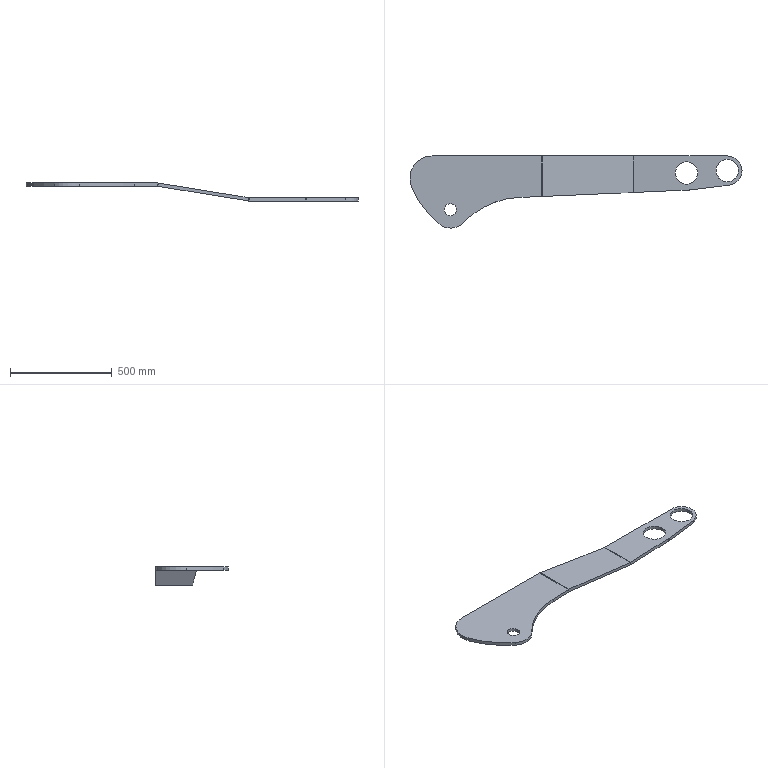Part | SolidWorks | features SM3dBend 2, FlatPattern 1, SMBaseFlange 1, SheetMetal 1 | 1 solid | 34 faces | box 1631 x 354.5 x 88.747 mm | volume 5017835 mm3 | cylinder 17 | plane 15 | spline 2 | commonest cylinder face diameters 60 x4 110 x4 28 x2 144 x2 168 x1 180 x1
STEP:
#1=CARTESIAN_POINT('',(1304.262,192.5,-88.747));
#2=VERTEX_POINT('',#1);
#3=CARTESIAN_POINT('',(1414.262,192.5,-88.747));
#4=VERTEX_POINT('',#3);
#5=CARTESIAN_POINT('',(1359.262,192.5,-88.747));
#6=DIRECTION('',(0.,0.,1.));
#7=DIRECTION('',(1.,0.,0.));
#8=AXIS2_PLACEMENT_3D('',#5,#6,#7);
#9=CIRCLE('',#8,55.);
#10=EDGE_CURVE('',#2,#4,#9,.T.);
#11=ORIENTED_EDGE('',*,*,#10,.F.);
#12=CARTESIAN_POINT('',(1304.262,192.5,-72.747));
#13=VERTEX_POINT('',#12);
#14=CARTESIAN_POINT('',(1304.262,192.5,-88.747));
#15=DIRECTION('',(0.,0.,1.));
#16=VECTOR('',#15,1000.);
#17=LINE('',#14,#16);
#18=EDGE_CURVE('',#2,#13,#17,.T.);
#19=ORIENTED_EDGE('',*,*,#18,.T.);
#20=CARTESIAN_POINT('',(1414.262,192.5,-72.747));
#21=VERTEX_POINT('',#20);
#22=CARTESIAN_POINT('',(1359.262,192.5,-72.747));
#23=DIRECTION('',(0.,0.,1.));
#24=DIRECTION('',(1.,0.,0.));
#25=AXIS2_PLACEMENT_3D('',#22,#23,#24);
#26=CIRCLE('',#25,55.);
#27=EDGE_CURVE('',#13,#21,#26,.T.);
#28=ORIENTED_EDGE('',*,*,#27,.T.);
#29=CARTESIAN_POINT('',(1414.262,192.5,-88.747));
#30=DIRECTION('',(0.,0.,1.));
#31=VECTOR('',#30,1000.);
#32=LINE('',#29,#31);
#33=EDGE_CURVE('',#4,#21,#32,.T.);
#34=ORIENTED_EDGE('',*,*,#33,.F.);
#35=EDGE_LOOP('',(#11,#19,#28,#34));
#36=FACE_OUTER_BOUND('',#35,.T.);
#37=CARTESIAN_POINT('',(1359.262,192.5,-88.747));
#38=DIRECTION('',(0.,0.,1.));
#39=DIRECTION('',(1.,0.,0.));
#40=AXIS2_PLACEMENT_3D('',#37,#38,#39);
#41=CYLINDRICAL_SURFACE('',#40,55.);
#42=ADVANCED_FACE('',(#36),#41,.F.);
#43=CARTESIAN_POINT('',(1104.262,180.5,-88.747));
#44=VERTEX_POINT('',#43);
#45=CARTESIAN_POINT('',(1214.262,180.5,-88.747));
#46=VERTEX_POINT('',#45);
#47=CARTESIAN_POINT('',(1159.262,180.5,-88.747));
#48=DIRECTION('',(0.,0.,1.));
#49=DIRECTION('',(1.,0.,0.));
#50=AXIS2_PLACEMENT_3D('',#47,#48,#49);
#51=CIRCLE('',#50,55.);
#52=EDGE_CURVE('',#44,#46,#51,.T.);
#53=ORIENTED_EDGE('',*,*,#52,.F.);
#54=CARTESIAN_POINT('',(1104.262,180.5,-72.747));
#55=VERTEX_POINT('',#54);
#56=CARTESIAN_POINT('',(1104.262,180.5,-88.747));
#57=DIRECTION('',(0.,0.,1.));
#58=VECTOR('',#57,1000.);
#59=LINE('',#56,#58);
#60=EDGE_CURVE('',#44,#55,#59,.T.);
#61=ORIENTED_EDGE('',*,*,#60,.T.);
#62=CARTESIAN_POINT('',(1214.262,180.5,-72.747));
#63=VERTEX_POINT('',#62);
#64=CARTESIAN_POINT('',(1159.262,180.5,-72.747));
#65=DIRECTION('',(0.,0.,1.));
#66=DIRECTION('',(1.,0.,0.));
#67=AXIS2_PLACEMENT_3D('',#64,#65,#66);
#68=CIRCLE('',#67,55.);
#69=EDGE_CURVE('',#55,#63,#68,.T.);
#70=ORIENTED_EDGE('',*,*,#69,.T.);
#71=CARTESIAN_POINT('',(1214.262,180.5,-88.747));
#72=DIRECTION('',(0.,0.,1.));
#73=VECTOR('',#72,1000.);
#74=LINE('',#71,#73);
#75=EDGE_CURVE('',#46,#63,#74,.T.);
#76=ORIENTED_EDGE('',*,*,#75,.F.);
#77=EDGE_LOOP('',(#53,#61,#70,#76));
#78=FACE_OUTER_BOUND('',#77,.T.);
#79=CARTESIAN_POINT('',(1159.262,180.5,-88.747));
#80=DIRECTION('',(0.,0.,1.));
#81=DIRECTION('',(1.,0.,0.));
#82=AXIS2_PLACEMENT_3D('',#79,#80,#81);
#83=CYLINDRICAL_SURFACE('',#82,55.);
#84=ADVANCED_FACE('',(#78),#83,.F.);
#85=CARTESIAN_POINT('',(1368.037,121.037,-88.747));
#86=VERTEX_POINT('',#85);
#87=CARTESIAN_POINT('',(1431.262,192.5,-88.747));
#88=VERTEX_POINT('',#87);
#89=CARTESIAN_POINT('',(1359.262,192.5,-88.747));
#90=DIRECTION('',(0.,0.,1.));
#91=DIRECTION('',(1.,0.,0.));
#92=AXIS2_PLACEMENT_3D('',#89,#90,#91);
#93=CIRCLE('',#92,72.);
#94=EDGE_CURVE('',#86,#88,#93,.T.);
#95=ORIENTED_EDGE('',*,*,#94,.T.);
#96=CARTESIAN_POINT('',(1431.262,192.5,-72.747));
#97=VERTEX_POINT('',#96);
#98=CARTESIAN_POINT('',(1431.262,192.5,-88.747));
#99=DIRECTION('',(0.,0.,1.));
#100=VECTOR('',#99,1000.);
#101=LINE('',#98,#100);
#102=EDGE_CURVE('',#88,#97,#101,.T.);
#103=ORIENTED_EDGE('',*,*,#102,.T.);
#104=CARTESIAN_POINT('',(1368.037,121.037,-72.747));
#105=VERTEX_POINT('',#104);
#106=CARTESIAN_POINT('',(1359.262,192.5,-72.747));
#107=DIRECTION('',(0.,0.,1.));
#108=DIRECTION('',(1.,0.,0.));
#109=AXIS2_PLACEMENT_3D('',#106,#107,#108);
#110=CIRCLE('',#109,72.);
#111=EDGE_CURVE('',#105,#97,#110,.T.);
#112=ORIENTED_EDGE('',*,*,#111,.F.);
#113=CARTESIAN_POINT('',(1368.037,121.037,-88.747));
#114=DIRECTION('',(0.,0.,1.));
#115=VECTOR('',#114,1000.);
#116=LINE('',#113,#115);
#117=EDGE_CURVE('',#86,#105,#116,.T.);
#118=ORIENTED_EDGE('',*,*,#117,.F.);
#119=EDGE_LOOP('',(#95,#103,#112,#118));
#120=FACE_OUTER_BOUND('',#119,.T.);
#121=CARTESIAN_POINT('',(1359.262,192.5,-88.747));
#122=DIRECTION('',(0.,0.,1.));
#123=DIRECTION('',(1.,0.,0.));
#124=AXIS2_PLACEMENT_3D('',#121,#122,#123);
#125=CYLINDRICAL_SURFACE('',#124,72.);
#126=ADVANCED_FACE('',(#120),#125,.T.);
#127=CARTESIAN_POINT('',(-30.,0.,-16.));
#128=VERTEX_POINT('',#127);
#129=CARTESIAN_POINT('',(30.,0.,-16.));
#130=VERTEX_POINT('',#129);
#131=CARTESIAN_POINT('',(0.,0.,-16.));
#132=DIRECTION('',(0.,0.,1.));
#133=DIRECTION('',(1.,0.,0.));
#134=AXIS2_PLACEMENT_3D('',#131,#132,#133);
#135=CIRCLE('',#134,30.);
#136=EDGE_CURVE('',#128,#130,#135,.T.);
#137=ORIENTED_EDGE('',*,*,#136,.F.);
#138=CARTESIAN_POINT('',(-30.,0.,0.));
#139=VERTEX_POINT('',#138);
#140=CARTESIAN_POINT('',(-30.,0.,-16.));
#141=DIRECTION('',(0.,0.,1.));
#142=VECTOR('',#141,1000.);
#143=LINE('',#140,#142);
#144=EDGE_CURVE('',#128,#139,#143,.T.);
#145=ORIENTED_EDGE('',*,*,#144,.T.);
#146=CARTESIAN_POINT('',(30.,0.,0.));
#147=VERTEX_POINT('',#146);
#148=CARTESIAN_POINT('',(0.,0.,0.));
#149=DIRECTION('',(0.,0.,1.));
#150=DIRECTION('',(1.,0.,0.));
#151=AXIS2_PLACEMENT_3D('',#148,#149,#150);
#152=CIRCLE('',#151,30.);
#153=EDGE_CURVE('',#139,#147,#152,.T.);
#154=ORIENTED_EDGE('',*,*,#153,.T.);
#155=CARTESIAN_POINT('',(30.,0.,-16.));
#156=DIRECTION('',(0.,0.,1.));
#157=VECTOR('',#156,1000.);
#158=LINE('',#155,#157);
#159=EDGE_CURVE('',#130,#147,#158,.T.);
#160=ORIENTED_EDGE('',*,*,#159,.F.);
#161=EDGE_LOOP('',(#137,#145,#154,#160));
#162=FACE_OUTER_BOUND('',#161,.T.);
#163=CARTESIAN_POINT('',(0.,0.,-16.));
#164=DIRECTION('',(0.,0.,1.));
#165=DIRECTION('',(1.,0.,0.));
#166=AXIS2_PLACEMENT_3D('',#163,#164,#165);
#167=CYLINDRICAL_SURFACE('',#166,30.);
#168=ADVANCED_FACE('',(#162),#167,.F.);
#169=CARTESIAN_POINT('',(896.39,264.5,-72.567));
#170=VERTEX_POINT('',#169);
#171=CARTESIAN_POINT('',(450.73,264.5,-0.3859));
#172=VERTEX_POINT('',#171);
#173=CARTESIAN_POINT('',(-82.093,264.5,85.913));
#174=DIRECTION('',(-0.9871,0.,0.1599));
#175=VECTOR('',#174,1000.);
#176=LINE('',#173,#175);
#177=EDGE_CURVE('',#170,#172,#176,.T.);
#178=ORIENTED_EDGE('',*,*,#177,.F.);
#179=CARTESIAN_POINT('',(893.832,264.5,-88.361));
#180=VERTEX_POINT('',#179);
#181=CARTESIAN_POINT('',(893.832,264.5,-88.361));
#182=DIRECTION('',(-0.1599,0.,-0.9871));
#183=VECTOR('',#182,1000.);
#184=LINE('',#181,#183);
#185=EDGE_CURVE('',#170,#180,#184,.T.);
#186=ORIENTED_EDGE('',*,*,#185,.T.);
#187=CARTESIAN_POINT('',(448.172,264.5,-16.18));
#188=VERTEX_POINT('',#187);
#189=CARTESIAN_POINT('',(-84.651,264.5,70.118));
#190=DIRECTION('',(-0.9871,0.,0.1599));
#191=VECTOR('',#190,1000.);
#192=LINE('',#189,#191);
#193=EDGE_CURVE('',#180,#188,#192,.T.);
#194=ORIENTED_EDGE('',*,*,#193,.T.);
#195=CARTESIAN_POINT('',(448.172,264.5,-16.18));
#196=DIRECTION('',(-0.1599,0.,-0.9871));
#197=VECTOR('',#196,1000.);
#198=LINE('',#195,#197);
#199=EDGE_CURVE('',#172,#188,#198,.T.);
#200=ORIENTED_EDGE('',*,*,#199,.F.);
#201=EDGE_LOOP('',(#178,#186,#194,#200));
#202=FACE_OUTER_BOUND('',#201,.T.);
#203=CARTESIAN_POINT('',(-84.651,264.5,70.118));
#204=DIRECTION('',(0.,1.,0.));
#205=DIRECTION('',(0.1599,0.,0.9871));
#206=AXIS2_PLACEMENT_3D('',#203,#204,#205);
#207=PLANE('',#206);
#208=ADVANCED_FACE('',(#202),#207,.T.);
#209=CARTESIAN_POINT('',(448.172,65.38,-16.18));
#210=VERTEX_POINT('',#209);
#211=CARTESIAN_POINT('',(893.832,85.091,-88.361));
#212=VERTEX_POINT('',#211);
#213=CARTESIAN_POINT('',(1166.601,97.156,-132.54));
#214=DIRECTION('',(0.9862,0.04362,-0.1597));
#215=VECTOR('',#214,1000.);
#216=LINE('',#213,#215);
#217=EDGE_CURVE('',#210,#212,#216,.T.);
#218=ORIENTED_EDGE('',*,*,#217,.T.);
#219=CARTESIAN_POINT('',(896.39,85.091,-72.567));
#220=VERTEX_POINT('',#219);
#221=CARTESIAN_POINT('',(893.832,85.091,-88.361));
#222=CARTESIAN_POINT('',(894.685,85.091,-83.097));
#223=CARTESIAN_POINT('',(895.537,85.091,-77.832));
#224=CARTESIAN_POINT('',(896.39,85.091,-72.567));
#225=B_SPLINE_CURVE_WITH_KNOTS('',3,(#221,#222,#223,#224),.UNSPECIFIED.,.F.,.F.,(4,4),(0.,1.),.UNSPECIFIED.);
#226=EDGE_CURVE('',#212,#220,#225,.T.);
#227=ORIENTED_EDGE('',*,*,#226,.T.);
#228=CARTESIAN_POINT('',(450.73,65.38,-0.3859));
#229=VERTEX_POINT('',#228);
#230=CARTESIAN_POINT('',(1169.159,97.156,-116.746));
#231=DIRECTION('',(0.9862,0.04362,-0.1597));
#232=VECTOR('',#231,1000.);
#233=LINE('',#230,#232);
#234=EDGE_CURVE('',#229,#220,#233,.T.);
#235=ORIENTED_EDGE('',*,*,#234,.F.);
#236=CARTESIAN_POINT('',(448.172,65.38,-16.18));
#237=CARTESIAN_POINT('',(450.73,65.38,-0.3859));
#238=B_SPLINE_CURVE_WITH_KNOTS('',1,(#236,#237),.UNSPECIFIED.,.F.,.F.,(2,2),(0.,1.),.UNSPECIFIED.);
#239=EDGE_CURVE('',#210,#229,#238,.T.);
#240=ORIENTED_EDGE('',*,*,#239,.F.);
#241=EDGE_LOOP('',(#218,#227,#235,#240));
#242=FACE_OUTER_BOUND('',#241,.T.);
#243=CARTESIAN_POINT('',(1166.601,97.156,-132.54));
#244=DIRECTION('',(0.04306,-0.999,-0.006974));
#245=DIRECTION('',(0.9862,0.04362,-0.1597));
#246=AXIS2_PLACEMENT_3D('',#243,#244,#245);
#247=PLANE('',#246);
#248=ADVANCED_FACE('',(#242),#247,.T.);
#249=ORIENTED_EDGE('',*,*,#234,.T.);
#250=CARTESIAN_POINT('',(896.39,155.5,-72.567));
#251=DIRECTION('',(0.,1.,0.));
#252=VECTOR('',#251,1000.);
#253=LINE('',#250,#252);
#254=EDGE_CURVE('',#220,#170,#253,.T.);
#255=ORIENTED_EDGE('',*,*,#254,.T.);
#256=ORIENTED_EDGE('',*,*,#177,.T.);
#257=CARTESIAN_POINT('',(450.73,155.5,-0.3859));
#258=DIRECTION('',(0.,1.,0.));
#259=VECTOR('',#258,1000.);
#260=LINE('',#257,#259);
#261=EDGE_CURVE('',#229,#172,#260,.T.);
#262=ORIENTED_EDGE('',*,*,#261,.F.);
#263=EDGE_LOOP('',(#249,#255,#256,#262));
#264=FACE_OUTER_BOUND('',#263,.T.);
#265=CARTESIAN_POINT('',(-82.093,155.5,85.913));
#266=DIRECTION('',(0.1599,0.,0.9871));
#267=DIRECTION('',(0.9871,0.,-0.1599));
#268=AXIS2_PLACEMENT_3D('',#265,#266,#267);
#269=PLANE('',#268);
#270=ADVANCED_FACE('',(#264),#269,.T.);
#271=CARTESIAN_POINT('',(893.832,155.5,-88.361));
#272=DIRECTION('',(0.,1.,0.));
#273=VECTOR('',#272,1000.);
#274=LINE('',#271,#273);
#275=EDGE_CURVE('',#212,#180,#274,.T.);
#276=ORIENTED_EDGE('',*,*,#275,.F.);
#277=ORIENTED_EDGE('',*,*,#217,.F.);
#278=CARTESIAN_POINT('',(448.172,155.5,-16.18));
#279=DIRECTION('',(0.,1.,0.));
#280=VECTOR('',#279,1000.);
#281=LINE('',#278,#280);
#282=EDGE_CURVE('',#210,#188,#281,.T.);
#283=ORIENTED_EDGE('',*,*,#282,.T.);
#284=ORIENTED_EDGE('',*,*,#193,.F.);
#285=EDGE_LOOP('',(#276,#277,#283,#284));
#286=FACE_OUTER_BOUND('',#285,.T.);
#287=CARTESIAN_POINT('',(-84.651,155.5,70.118));
#288=DIRECTION('',(0.1599,0.,0.9871));
#289=DIRECTION('',(0.9871,0.,-0.1599));
#290=AXIS2_PLACEMENT_3D('',#287,#288,#289);
#291=PLANE('',#290);
#292=ADVANCED_FACE('',(#286),#291,.F.);
#293=ORIENTED_EDGE('',*,*,#144,.F.);
#294=CARTESIAN_POINT('',(0.,0.,-16.));
#295=DIRECTION('',(0.,0.,1.));
#296=DIRECTION('',(1.,0.,0.));
#297=AXIS2_PLACEMENT_3D('',#294,#295,#296);
#298=CIRCLE('',#297,30.);
#299=EDGE_CURVE('',#130,#128,#298,.T.);
#300=ORIENTED_EDGE('',*,*,#299,.F.);
#301=ORIENTED_EDGE('',*,*,#159,.T.);
#302=CARTESIAN_POINT('',(0.,0.,0.));
#303=DIRECTION('',(0.,0.,1.));
#304=DIRECTION('',(1.,0.,0.));
#305=AXIS2_PLACEMENT_3D('',#302,#303,#304);
#306=CIRCLE('',#305,30.);
#307=EDGE_CURVE('',#147,#139,#306,.T.);
#308=ORIENTED_EDGE('',*,*,#307,.T.);
#309=EDGE_LOOP('',(#293,#300,#301,#308));
#310=FACE_OUTER_BOUND('',#309,.T.);
#311=CARTESIAN_POINT('',(0.,0.,-16.));
#312=DIRECTION('',(0.,0.,1.));
#313=DIRECTION('',(1.,0.,0.));
#314=AXIS2_PLACEMENT_3D('',#311,#312,#313);
#315=CYLINDRICAL_SURFACE('',#314,30.);
#316=ADVANCED_FACE('',(#310),#315,.F.);
#317=CARTESIAN_POINT('',(-90.3,264.5,0.));
#318=VERTEX_POINT('',#317);
#319=CARTESIAN_POINT('',(-191.607,115.278,0.));
#320=VERTEX_POINT('',#319);
#321=CARTESIAN_POINT('',(-90.3,155.5,0.));
#322=DIRECTION('',(0.,0.,1.));
#323=DIRECTION('',(1.,0.,0.));
#324=AXIS2_PLACEMENT_3D('',#321,#322,#323);
#325=CIRCLE('',#324,109.);
#326=EDGE_CURVE('',#318,#320,#325,.T.);
#327=ORIENTED_EDGE('',*,*,#326,.F.);
#328=CARTESIAN_POINT('',(-90.3,264.5,-16.));
#329=VERTEX_POINT('',#328);
#330=CARTESIAN_POINT('',(-90.3,264.5,-16.));
#331=DIRECTION('',(0.,0.,1.));
#332=VECTOR('',#331,1000.);
#333=LINE('',#330,#332);
#334=EDGE_CURVE('',#329,#318,#333,.T.);
#335=ORIENTED_EDGE('',*,*,#334,.F.);
#336=CARTESIAN_POINT('',(-191.607,115.278,-16.));
#337=VERTEX_POINT('',#336);
#338=CARTESIAN_POINT('',(-90.3,155.5,-16.));
#339=DIRECTION('',(0.,0.,1.));
#340=DIRECTION('',(1.,0.,0.));
#341=AXIS2_PLACEMENT_3D('',#338,#339,#340);
#342=CIRCLE('',#341,109.);
#343=EDGE_CURVE('',#329,#337,#342,.T.);
#344=ORIENTED_EDGE('',*,*,#343,.T.);
#345=CARTESIAN_POINT('',(-191.607,115.278,-16.));
#346=DIRECTION('',(0.,0.,1.));
#347=VECTOR('',#346,1000.);
#348=LINE('',#345,#347);
#349=EDGE_CURVE('',#337,#320,#348,.T.);
#350=ORIENTED_EDGE('',*,*,#349,.T.);
#351=EDGE_LOOP('',(#327,#335,#344,#350));
#352=FACE_OUTER_BOUND('',#351,.T.);
#353=CARTESIAN_POINT('',(-90.3,155.5,-16.));
#354=DIRECTION('',(0.,0.,1.));
#355=DIRECTION('',(1.,0.,0.));
#356=AXIS2_PLACEMENT_3D('',#353,#354,#355);
#357=CYLINDRICAL_SURFACE('',#356,109.);
#358=ADVANCED_FACE('',(#352),#357,.T.);
#359=CARTESIAN_POINT('',(-57.388,-69.33,0.));
#360=VERTEX_POINT('',#359);
#361=CARTESIAN_POINT('',(235.928,285.022,0.));
#362=DIRECTION('',(0.,0.,1.));
#363=DIRECTION('',(1.,0.,0.));
#364=AXIS2_PLACEMENT_3D('',#361,#362,#363);
#365=CIRCLE('',#364,460.);
#366=EDGE_CURVE('',#320,#360,#365,.T.);
#367=ORIENTED_EDGE('',*,*,#366,.F.);
#368=ORIENTED_EDGE('',*,*,#349,.F.);
#369=CARTESIAN_POINT('',(-57.388,-69.33,-16.));
#370=VERTEX_POINT('',#369);
#371=CARTESIAN_POINT('',(235.928,285.022,-16.));
#372=DIRECTION('',(0.,0.,1.));
#373=DIRECTION('',(1.,0.,0.));
#374=AXIS2_PLACEMENT_3D('',#371,#372,#373);
#375=CIRCLE('',#374,460.);
#376=EDGE_CURVE('',#337,#370,#375,.T.);
#377=ORIENTED_EDGE('',*,*,#376,.T.);
#378=CARTESIAN_POINT('',(-57.388,-69.33,-16.));
#379=DIRECTION('',(0.,0.,1.));
#380=VECTOR('',#379,1000.);
#381=LINE('',#378,#380);
#382=EDGE_CURVE('',#370,#360,#381,.T.);
#383=ORIENTED_EDGE('',*,*,#382,.T.);
#384=EDGE_LOOP('',(#367,#368,#377,#383));
#385=FACE_OUTER_BOUND('',#384,.T.);
#386=CARTESIAN_POINT('',(235.928,285.022,-16.));
#387=DIRECTION('',(0.,0.,1.));
#388=DIRECTION('',(1.,0.,0.));
#389=AXIS2_PLACEMENT_3D('',#386,#387,#388);
#390=CYLINDRICAL_SURFACE('',#389,460.);
#391=ADVANCED_FACE('',(#385),#390,.T.);
#392=CARTESIAN_POINT('',(64.952,-62.299,0.));
#393=VERTEX_POINT('',#392);
#394=CARTESIAN_POINT('',(0.,0.,0.));
#395=DIRECTION('',(0.,0.,1.));
#396=DIRECTION('',(1.,0.,0.));
#397=AXIS2_PLACEMENT_3D('',#394,#395,#396);
#398=CIRCLE('',#397,90.);
#399=EDGE_CURVE('',#360,#393,#398,.T.);
#400=ORIENTED_EDGE('',*,*,#399,.F.);
#401=ORIENTED_EDGE('',*,*,#382,.F.);
#402=CARTESIAN_POINT('',(64.952,-62.299,-16.));
#403=VERTEX_POINT('',#402);
#404=CARTESIAN_POINT('',(0.,0.,-16.));
#405=DIRECTION('',(0.,0.,1.));
#406=DIRECTION('',(1.,0.,0.));
#407=AXIS2_PLACEMENT_3D('',#404,#405,#406);
#408=CIRCLE('',#407,90.);
#409=EDGE_CURVE('',#370,#403,#408,.T.);
#410=ORIENTED_EDGE('',*,*,#409,.T.);
#411=CARTESIAN_POINT('',(64.952,-62.299,-16.));
#412=DIRECTION('',(0.,0.,1.));
#413=VECTOR('',#412,1000.);
#414=LINE('',#411,#413);
#415=EDGE_CURVE('',#403,#393,#414,.T.);
#416=ORIENTED_EDGE('',*,*,#415,.T.);
#417=EDGE_LOOP('',(#400,#401,#410,#416));
#418=FACE_OUTER_BOUND('',#417,.T.);
#419=CARTESIAN_POINT('',(0.,0.,-16.));
#420=DIRECTION('',(0.,0.,1.));
#421=DIRECTION('',(1.,0.,0.));
#422=AXIS2_PLACEMENT_3D('',#419,#420,#421);
#423=CYLINDRICAL_SURFACE('',#422,90.);
#424=ADVANCED_FACE('',(#418),#423,.T.);
#425=CARTESIAN_POINT('',(336.181,60.434,0.));
#426=VERTEX_POINT('',#425);
#427=CARTESIAN_POINT('',(353.629,-339.185,0.));
#428=DIRECTION('',(0.,0.,-1.));
#429=DIRECTION('',(1.,0.,0.));
#430=AXIS2_PLACEMENT_3D('',#427,#428,#429);
#431=CIRCLE('',#430,400.);
#432=EDGE_CURVE('',#393,#426,#431,.T.);
#433=ORIENTED_EDGE('',*,*,#432,.F.);
#434=ORIENTED_EDGE('',*,*,#415,.F.);
#435=CARTESIAN_POINT('',(336.181,60.434,-16.));
#436=VERTEX_POINT('',#435);
#437=CARTESIAN_POINT('',(353.629,-339.185,-16.));
#438=DIRECTION('',(0.,0.,-1.));
#439=DIRECTION('',(1.,0.,0.));
#440=AXIS2_PLACEMENT_3D('',#437,#438,#439);
#441=CIRCLE('',#440,400.);
#442=EDGE_CURVE('',#403,#436,#441,.T.);
#443=ORIENTED_EDGE('',*,*,#442,.T.);
#444=CARTESIAN_POINT('',(336.181,60.434,-16.));
#445=DIRECTION('',(0.,0.,1.));
#446=VECTOR('',#445,1000.);
#447=LINE('',#444,#446);
#448=EDGE_CURVE('',#436,#426,#447,.T.);
#449=ORIENTED_EDGE('',*,*,#448,.T.);
#450=EDGE_LOOP('',(#433,#434,#443,#449));
#451=FACE_OUTER_BOUND('',#450,.T.);
#452=CARTESIAN_POINT('',(353.629,-339.185,-16.));
#453=DIRECTION('',(0.,0.,1.));
#454=DIRECTION('',(1.,0.,0.));
#455=AXIS2_PLACEMENT_3D('',#452,#453,#454);
#456=CYLINDRICAL_SURFACE('',#455,400.);
#457=ADVANCED_FACE('',(#451),#456,.F.);
#458=CARTESIAN_POINT('',(445.934,65.226,-16.));
#459=VERTEX_POINT('',#458);
#460=CARTESIAN_POINT('',(445.934,264.5,-16.));
#461=VERTEX_POINT('',#460);
#462=CARTESIAN_POINT('',(445.934,155.5,-16.));
#463=DIRECTION('',(0.,1.,0.));
#464=VECTOR('',#463,1000.);
#465=LINE('',#462,#464);
#466=EDGE_CURVE('',#459,#461,#465,.T.);
#467=ORIENTED_EDGE('',*,*,#466,.F.);
#468=CARTESIAN_POINT('',(1177.258,97.156,-16.));
#469=DIRECTION('',(0.999,0.04362,0.));
#470=VECTOR('',#469,1000.);
#471=LINE('',#468,#470);
#472=EDGE_CURVE('',#436,#459,#471,.T.);
#473=ORIENTED_EDGE('',*,*,#472,.F.);
#474=ORIENTED_EDGE('',*,*,#442,.F.);
#475=ORIENTED_EDGE('',*,*,#409,.F.);
#476=ORIENTED_EDGE('',*,*,#376,.F.);
#477=ORIENTED_EDGE('',*,*,#343,.F.);
#478=CARTESIAN_POINT('',(-90.3,264.5,-16.));
#479=DIRECTION('',(-1.,0.,0.));
#480=VECTOR('',#479,1000.);
#481=LINE('',#478,#480);
#482=EDGE_CURVE('',#461,#329,#481,.T.);
#483=ORIENTED_EDGE('',*,*,#482,.F.);
#484=EDGE_LOOP('',(#467,#473,#474,#475,#476,#477,#483));
#485=FACE_OUTER_BOUND('',#484,.T.);
#486=ORIENTED_EDGE('',*,*,#299,.T.);
#487=ORIENTED_EDGE('',*,*,#136,.T.);
#488=EDGE_LOOP('',(#486,#487));
#489=FACE_BOUND('',#488,.T.);
#490=CARTESIAN_POINT('',(-90.3,155.5,-16.));
#491=DIRECTION('',(0.,0.,1.));
#492=DIRECTION('',(1.,0.,0.));
#493=AXIS2_PLACEMENT_3D('',#490,#491,#492);
#494=PLANE('',#493);
#495=ADVANCED_FACE('',(#485,#489),#494,.F.);
#496=ORIENTED_EDGE('',*,*,#472,.T.);
#497=CARTESIAN_POINT('',(445.934,65.226,0.));
#498=VERTEX_POINT('',#497);
#499=CARTESIAN_POINT('',(445.934,65.226,-16.));
#500=CARTESIAN_POINT('',(445.934,65.226,-10.667));
#501=CARTESIAN_POINT('',(445.934,65.226,-5.333));
#502=CARTESIAN_POINT('',(445.934,65.226,0.));
#503=B_SPLINE_CURVE_WITH_KNOTS('',3,(#499,#500,#501,#502),.UNSPECIFIED.,.F.,.F.,(4,4),(0.,1.),.UNSPECIFIED.);
#504=EDGE_CURVE('',#459,#498,#503,.T.);
#505=ORIENTED_EDGE('',*,*,#504,.T.);
#506=CARTESIAN_POINT('',(1177.258,97.156,0.));
#507=DIRECTION('',(0.999,0.04362,0.));
#508=VECTOR('',#507,1000.);
#509=LINE('',#506,#508);
#510=EDGE_CURVE('',#426,#498,#509,.T.);
#511=ORIENTED_EDGE('',*,*,#510,.F.);
#512=ORIENTED_EDGE('',*,*,#448,.F.);
#513=EDGE_LOOP('',(#496,#505,#511,#512));
#514=FACE_OUTER_BOUND('',#513,.T.);
#515=CARTESIAN_POINT('',(1177.258,97.156,-16.));
#516=DIRECTION('',(0.04362,-0.999,0.));
#517=DIRECTION('',(0.999,0.04362,0.));
#518=AXIS2_PLACEMENT_3D('',#515,#516,#517);
#519=PLANE('',#518);
#520=ADVANCED_FACE('',(#514),#519,.T.);
#521=ORIENTED_EDGE('',*,*,#307,.F.);
#522=ORIENTED_EDGE('',*,*,#153,.F.);
#523=EDGE_LOOP('',(#521,#522));
#524=FACE_BOUND('',#523,.T.);
#525=ORIENTED_EDGE('',*,*,#510,.T.);
#526=CARTESIAN_POINT('',(445.934,264.5,0.));
#527=VERTEX_POINT('',#526);
#528=CARTESIAN_POINT('',(445.934,155.5,0.));
#529=DIRECTION('',(0.,1.,0.));
#530=VECTOR('',#529,1000.);
#531=LINE('',#528,#530);
#532=EDGE_CURVE('',#498,#527,#531,.T.);
#533=ORIENTED_EDGE('',*,*,#532,.T.);
#534=CARTESIAN_POINT('',(-90.3,264.5,0.));
#535=DIRECTION('',(-1.,0.,0.));
#536=VECTOR('',#535,1000.);
#537=LINE('',#534,#536);
#538=EDGE_CURVE('',#527,#318,#537,.T.);
#539=ORIENTED_EDGE('',*,*,#538,.T.);
#540=ORIENTED_EDGE('',*,*,#326,.T.);
#541=ORIENTED_EDGE('',*,*,#366,.T.);
#542=ORIENTED_EDGE('',*,*,#399,.T.);
#543=ORIENTED_EDGE('',*,*,#432,.T.);
#544=EDGE_LOOP('',(#525,#533,#539,#540,#541,#542,#543));
#545=FACE_OUTER_BOUND('',#544,.T.);
#546=CARTESIAN_POINT('',(-90.3,155.5,0.));
#547=DIRECTION('',(0.,0.,1.));
#548=DIRECTION('',(1.,0.,0.));
#549=AXIS2_PLACEMENT_3D('',#546,#547,#548);
#550=PLANE('',#549);
#551=ADVANCED_FACE('',(#524,#545),#550,.T.);
#552=ORIENTED_EDGE('',*,*,#538,.F.);
#553=CARTESIAN_POINT('',(445.934,264.5,-16.));
#554=DIRECTION('',(0.,0.,-1.));
#555=VECTOR('',#554,1000.);
#556=LINE('',#553,#555);
#557=EDGE_CURVE('',#527,#461,#556,.T.);
#558=ORIENTED_EDGE('',*,*,#557,.T.);
#559=ORIENTED_EDGE('',*,*,#482,.T.);
#560=ORIENTED_EDGE('',*,*,#334,.T.);
#561=EDGE_LOOP('',(#552,#558,#559,#560));
#562=FACE_OUTER_BOUND('',#561,.T.);
#563=CARTESIAN_POINT('',(-90.3,264.5,-16.));
#564=DIRECTION('',(0.,1.,0.));
#565=DIRECTION('',(0.,0.,1.));
#566=AXIS2_PLACEMENT_3D('',#563,#564,#565);
#567=PLANE('',#566);
#568=ADVANCED_FACE('',(#562),#567,.T.);
#569=ORIENTED_EDGE('',*,*,#239,.T.);
#570=CARTESIAN_POINT('',(450.73,65.38,-0.3859));
#571=CARTESIAN_POINT('',(449.145,65.329,-0.1292));
#572=CARTESIAN_POINT('',(447.539,65.277,0.));
#573=CARTESIAN_POINT('',(445.934,65.226,0.));
#574=B_SPLINE_CURVE_WITH_KNOTS('',3,(#570,#571,#572,#573),.UNSPECIFIED.,.F.,.F.,(4,4),(0.,1.),.UNSPECIFIED.);
#575=EDGE_CURVE('',#229,#498,#574,.T.);
#576=ORIENTED_EDGE('',*,*,#575,.T.);
#577=ORIENTED_EDGE('',*,*,#504,.F.);
#578=CARTESIAN_POINT('',(448.172,65.38,-16.18));
#579=CARTESIAN_POINT('',(447.432,65.329,-16.06));
#580=CARTESIAN_POINT('',(446.683,65.277,-16.));
#581=CARTESIAN_POINT('',(445.934,65.226,-16.));
#582=B_SPLINE_CURVE_WITH_KNOTS('',3,(#578,#579,#580,#581),.UNSPECIFIED.,.F.,.F.,(4,4),(0.,1.),.UNSPECIFIED.);
#583=EDGE_CURVE('',#210,#459,#582,.T.);
#584=ORIENTED_EDGE('',*,*,#583,.F.);
#585=EDGE_LOOP('',(#569,#576,#577,#584));
#586=FACE_OUTER_BOUND('',#585,.T.);
#587=CARTESIAN_POINT('',(450.73,65.38,-0.3859));
#588=CARTESIAN_POINT('',(449.145,65.329,-0.1292));
#589=CARTESIAN_POINT('',(447.539,65.277,0.));
#590=CARTESIAN_POINT('',(445.934,65.226,0.));
#591=CARTESIAN_POINT('',(448.172,65.38,-16.18));
#592=CARTESIAN_POINT('',(447.432,65.329,-16.06));
#593=CARTESIAN_POINT('',(446.683,65.277,-16.));
#594=CARTESIAN_POINT('',(445.934,65.226,-16.));
#595=B_SPLINE_SURFACE_WITH_KNOTS('',1,3,((#587,#588,#589,#590),(#591,#592,#593,#594)),.UNSPECIFIED.,.F.,.F.,.F.,(2,2),(4,4),(0.,1.),(0.,1.),.UNSPECIFIED.);
#596=ADVANCED_FACE('',(#586),#595,.F.);
#597=ORIENTED_EDGE('',*,*,#557,.F.);
#598=CARTESIAN_POINT('',(445.934,264.5,-30.));
#599=DIRECTION('',(0.,1.,0.));
#600=DIRECTION('',(1.,0.,0.));
#601=AXIS2_PLACEMENT_3D('',#598,#599,#600);
#602=CIRCLE('',#601,30.);
#603=EDGE_CURVE('',#527,#172,#602,.T.);
#604=ORIENTED_EDGE('',*,*,#603,.T.);
#605=ORIENTED_EDGE('',*,*,#199,.T.);
#606=CARTESIAN_POINT('',(445.934,264.5,-30.));
#607=DIRECTION('',(0.,1.,0.));
#608=DIRECTION('',(0.,0.,-1.));
#609=AXIS2_PLACEMENT_3D('',#606,#607,#608);
#610=CIRCLE('',#609,14.);
#611=EDGE_CURVE('',#461,#188,#610,.T.);
#612=ORIENTED_EDGE('',*,*,#611,.F.);
#613=EDGE_LOOP('',(#597,#604,#605,#612));
#614=FACE_OUTER_BOUND('',#613,.T.);
#615=CARTESIAN_POINT('',(445.934,264.5,-30.));
#616=DIRECTION('',(0.,-1.,0.));
#617=DIRECTION('',(0.,0.,-1.));
#618=AXIS2_PLACEMENT_3D('',#615,#616,#617);
#619=PLANE('',#618);
#620=ADVANCED_FACE('',(#614),#619,.F.);
#621=ORIENTED_EDGE('',*,*,#611,.T.);
#622=ORIENTED_EDGE('',*,*,#282,.F.);
#623=ORIENTED_EDGE('',*,*,#583,.T.);
#624=ORIENTED_EDGE('',*,*,#466,.T.);
#625=EDGE_LOOP('',(#621,#622,#623,#624));
#626=FACE_OUTER_BOUND('',#625,.T.);
#627=CARTESIAN_POINT('',(445.934,364.81,-30.));
#628=DIRECTION('',(0.,-1.,0.));
#629=DIRECTION('',(1.,0.,0.));
#630=AXIS2_PLACEMENT_3D('',#627,#628,#629);
#631=CYLINDRICAL_SURFACE('',#630,14.);
#632=ADVANCED_FACE('',(#626),#631,.F.);
#633=ORIENTED_EDGE('',*,*,#603,.F.);
#634=ORIENTED_EDGE('',*,*,#532,.F.);
#635=ORIENTED_EDGE('',*,*,#575,.F.);
#636=ORIENTED_EDGE('',*,*,#261,.T.);
#637=EDGE_LOOP('',(#633,#634,#635,#636));
#638=FACE_OUTER_BOUND('',#637,.T.);
#639=CARTESIAN_POINT('',(445.934,364.81,-30.));
#640=DIRECTION('',(0.,-1.,0.));
#641=DIRECTION('',(1.,0.,0.));
#642=AXIS2_PLACEMENT_3D('',#639,#640,#641);
#643=CYLINDRICAL_SURFACE('',#642,30.);
#644=ADVANCED_FACE('',(#638),#643,.T.);
#645=CARTESIAN_POINT('',(898.628,85.246,-88.747));
#646=VERTEX_POINT('',#645);
#647=CARTESIAN_POINT('',(898.628,85.246,-72.747));
#648=VERTEX_POINT('',#647);
#649=CARTESIAN_POINT('',(898.628,85.246,-88.747));
#650=CARTESIAN_POINT('',(898.628,85.246,-72.747));
#651=B_SPLINE_CURVE_WITH_KNOTS('',1,(#649,#650),.UNSPECIFIED.,.F.,.F.,(2,2),(0.,1.),.UNSPECIFIED.);
#652=EDGE_CURVE('',#646,#648,#651,.T.);
#653=ORIENTED_EDGE('',*,*,#652,.T.);
#654=CARTESIAN_POINT('',(898.628,85.246,-72.747));
#655=CARTESIAN_POINT('',(897.879,85.194,-72.747));
#656=CARTESIAN_POINT('',(897.13,85.143,-72.687));
#657=CARTESIAN_POINT('',(896.39,85.091,-72.567));
#658=B_SPLINE_CURVE_WITH_KNOTS('',3,(#654,#655,#656,#657),.UNSPECIFIED.,.F.,.F.,(4,4),(0.,1.),.UNSPECIFIED.);
#659=EDGE_CURVE('',#648,#220,#658,.T.);
#660=ORIENTED_EDGE('',*,*,#659,.T.);
#661=ORIENTED_EDGE('',*,*,#226,.F.);
#662=CARTESIAN_POINT('',(898.628,85.246,-88.747));
#663=CARTESIAN_POINT('',(897.023,85.194,-88.747));
#664=CARTESIAN_POINT('',(895.417,85.143,-88.618));
#665=CARTESIAN_POINT('',(893.832,85.091,-88.361));
#666=B_SPLINE_CURVE_WITH_KNOTS('',3,(#662,#663,#664,#665),.UNSPECIFIED.,.F.,.F.,(4,4),(0.,1.),.UNSPECIFIED.);
#667=EDGE_CURVE('',#646,#212,#666,.T.);
#668=ORIENTED_EDGE('',*,*,#667,.F.);
#669=EDGE_LOOP('',(#653,#660,#661,#668));
#670=FACE_OUTER_BOUND('',#669,.T.);
#671=CARTESIAN_POINT('',(898.628,85.246,-88.747));
#672=CARTESIAN_POINT('',(897.023,85.194,-88.747));
#673=CARTESIAN_POINT('',(895.417,85.143,-88.618));
#674=CARTESIAN_POINT('',(893.832,85.091,-88.361));
#675=CARTESIAN_POINT('',(898.628,85.246,-72.747));
#676=CARTESIAN_POINT('',(897.879,85.194,-72.747));
#677=CARTESIAN_POINT('',(897.13,85.143,-72.687));
#678=CARTESIAN_POINT('',(896.39,85.091,-72.567));
#679=B_SPLINE_SURFACE_WITH_KNOTS('',1,3,((#671,#672,#673,#674),(#675,#676,#677,#678)),.UNSPECIFIED.,.F.,.F.,.F.,(2,2),(4,4),(0.,1.),(0.,1.),.UNSPECIFIED.);
#680=ADVANCED_FACE('',(#670),#679,.T.);
#681=ORIENTED_EDGE('',*,*,#185,.F.);
#682=CARTESIAN_POINT('',(898.628,264.5,-72.747));
#683=VERTEX_POINT('',#682);
#684=CARTESIAN_POINT('',(898.628,264.5,-58.747));
#685=DIRECTION('',(0.,-1.,0.));
#686=DIRECTION('',(1.,0.,0.));
#687=AXIS2_PLACEMENT_3D('',#684,#685,#686);
#688=CIRCLE('',#687,14.);
#689=EDGE_CURVE('',#170,#683,#688,.T.);
#690=ORIENTED_EDGE('',*,*,#689,.T.);
#691=CARTESIAN_POINT('',(898.628,264.5,-88.747));
#692=VERTEX_POINT('',#691);
#693=CARTESIAN_POINT('',(898.628,264.5,-88.747));
#694=DIRECTION('',(0.,0.,-1.));
#695=VECTOR('',#694,1000.);
#696=LINE('',#693,#695);
#697=EDGE_CURVE('',#683,#692,#696,.T.);
#698=ORIENTED_EDGE('',*,*,#697,.T.);
#699=CARTESIAN_POINT('',(898.628,264.5,-58.747));
#700=DIRECTION('',(0.,-1.,0.));
#701=DIRECTION('',(0.,0.,1.));
#702=AXIS2_PLACEMENT_3D('',#699,#700,#701);
#703=CIRCLE('',#702,30.);
#704=EDGE_CURVE('',#180,#692,#703,.T.);
#705=ORIENTED_EDGE('',*,*,#704,.F.);
#706=EDGE_LOOP('',(#681,#690,#698,#705));
#707=FACE_OUTER_BOUND('',#706,.T.);
#708=CARTESIAN_POINT('',(898.628,264.5,-58.747));
#709=DIRECTION('',(0.,1.,0.));
#710=DIRECTION('',(0.,0.,1.));
#711=AXIS2_PLACEMENT_3D('',#708,#709,#710);
#712=PLANE('',#711);
#713=ADVANCED_FACE('',(#707),#712,.T.);
#714=ORIENTED_EDGE('',*,*,#704,.T.);
#715=CARTESIAN_POINT('',(898.628,155.5,-88.747));
#716=DIRECTION('',(0.,1.,0.));
#717=VECTOR('',#716,1000.);
#718=LINE('',#715,#717);
#719=EDGE_CURVE('',#646,#692,#718,.T.);
#720=ORIENTED_EDGE('',*,*,#719,.F.);
#721=ORIENTED_EDGE('',*,*,#667,.T.);
#722=ORIENTED_EDGE('',*,*,#275,.T.);
#723=EDGE_LOOP('',(#714,#720,#721,#722));
#724=FACE_OUTER_BOUND('',#723,.T.);
#725=CARTESIAN_POINT('',(898.628,355.05,-58.747));
#726=DIRECTION('',(0.,-1.,0.));
#727=DIRECTION('',(1.,0.,0.));
#728=AXIS2_PLACEMENT_3D('',#725,#726,#727);
#729=CYLINDRICAL_SURFACE('',#728,30.);
#730=ADVANCED_FACE('',(#724),#729,.T.);
#731=ORIENTED_EDGE('',*,*,#689,.F.);
#732=ORIENTED_EDGE('',*,*,#254,.F.);
#733=ORIENTED_EDGE('',*,*,#659,.F.);
#734=CARTESIAN_POINT('',(898.628,155.5,-72.747));
#735=DIRECTION('',(0.,1.,0.));
#736=VECTOR('',#735,1000.);
#737=LINE('',#734,#736);
#738=EDGE_CURVE('',#648,#683,#737,.T.);
#739=ORIENTED_EDGE('',*,*,#738,.T.);
#740=EDGE_LOOP('',(#731,#732,#733,#739));
#741=FACE_OUTER_BOUND('',#740,.T.);
#742=CARTESIAN_POINT('',(898.628,355.05,-58.747));
#743=DIRECTION('',(0.,-1.,0.));
#744=DIRECTION('',(1.,0.,0.));
#745=AXIS2_PLACEMENT_3D('',#742,#743,#744);
#746=CYLINDRICAL_SURFACE('',#745,14.);
#747=ADVANCED_FACE('',(#741),#746,.F.);
#748=CARTESIAN_POINT('',(1171.42,97.156,-72.747));
#749=VERTEX_POINT('',#748);
#750=CARTESIAN_POINT('',(1177.993,97.702,-72.747));
#751=VERTEX_POINT('',#750);
#752=CARTESIAN_POINT('',(1167.756,181.076,-72.747));
#753=DIRECTION('',(0.,0.,1.));
#754=DIRECTION('',(1.,0.,0.));
#755=AXIS2_PLACEMENT_3D('',#752,#753,#754);
#756=CIRCLE('',#755,84.);
#757=EDGE_CURVE('',#749,#751,#756,.T.);
#758=ORIENTED_EDGE('',*,*,#757,.F.);
#759=CARTESIAN_POINT('',(1171.42,97.156,-88.747));
#760=VERTEX_POINT('',#759);
#761=CARTESIAN_POINT('',(1171.42,97.156,-88.747));
#762=DIRECTION('',(0.,0.,1.));
#763=VECTOR('',#762,1000.);
#764=LINE('',#761,#763);
#765=EDGE_CURVE('',#760,#749,#764,.T.);
#766=ORIENTED_EDGE('',*,*,#765,.F.);
#767=CARTESIAN_POINT('',(1177.993,97.702,-88.747));
#768=VERTEX_POINT('',#767);
#769=CARTESIAN_POINT('',(1167.756,181.076,-88.747));
#770=DIRECTION('',(0.,0.,1.));
#771=DIRECTION('',(1.,0.,0.));
#772=AXIS2_PLACEMENT_3D('',#769,#770,#771);
#773=CIRCLE('',#772,84.);
#774=EDGE_CURVE('',#760,#768,#773,.T.);
#775=ORIENTED_EDGE('',*,*,#774,.T.);
#776=CARTESIAN_POINT('',(1177.993,97.702,-88.747));
#777=DIRECTION('',(0.,0.,1.));
#778=VECTOR('',#777,1000.);
#779=LINE('',#776,#778);
#780=EDGE_CURVE('',#768,#751,#779,.T.);
#781=ORIENTED_EDGE('',*,*,#780,.T.);
#782=EDGE_LOOP('',(#758,#766,#775,#781));
#783=FACE_OUTER_BOUND('',#782,.T.);
#784=CARTESIAN_POINT('',(1167.756,181.076,-88.747));
#785=DIRECTION('',(0.,0.,1.));
#786=DIRECTION('',(1.,0.,0.));
#787=AXIS2_PLACEMENT_3D('',#784,#785,#786);
#788=CYLINDRICAL_SURFACE('',#787,84.);
#789=ADVANCED_FACE('',(#783),#788,.T.);
#790=CARTESIAN_POINT('',(1368.037,121.037,-72.747));
#791=DIRECTION('',(0.9925,0.1219,0.));
#792=VECTOR('',#791,1000.);
#793=LINE('',#790,#792);
#794=EDGE_CURVE('',#751,#105,#793,.T.);
#795=ORIENTED_EDGE('',*,*,#794,.F.);
#796=ORIENTED_EDGE('',*,*,#780,.F.);
#797=CARTESIAN_POINT('',(1368.037,121.037,-88.747));
#798=DIRECTION('',(0.9925,0.1219,0.));
#799=VECTOR('',#798,1000.);
#800=LINE('',#797,#799);
#801=EDGE_CURVE('',#768,#86,#800,.T.);
#802=ORIENTED_EDGE('',*,*,#801,.T.);
#803=ORIENTED_EDGE('',*,*,#117,.T.);
#804=EDGE_LOOP('',(#795,#796,#802,#803));
#805=FACE_OUTER_BOUND('',#804,.T.);
#806=CARTESIAN_POINT('',(1368.037,121.037,-88.747));
#807=DIRECTION('',(0.1219,-0.9925,0.));
#808=DIRECTION('',(0.9925,0.1219,0.));
#809=AXIS2_PLACEMENT_3D('',#806,#807,#808);
#810=PLANE('',#809);
#811=ADVANCED_FACE('',(#805),#810,.T.);
#812=ORIENTED_EDGE('',*,*,#102,.F.);
#813=CARTESIAN_POINT('',(1359.262,264.5,-88.747));
#814=VERTEX_POINT('',#813);
#815=CARTESIAN_POINT('',(1359.262,192.5,-88.747));
#816=DIRECTION('',(0.,0.,1.));
#817=DIRECTION('',(1.,0.,0.));
#818=AXIS2_PLACEMENT_3D('',#815,#816,#817);
#819=CIRCLE('',#818,72.);
#820=EDGE_CURVE('',#88,#814,#819,.T.);
#821=ORIENTED_EDGE('',*,*,#820,.T.);
#822=CARTESIAN_POINT('',(1359.262,264.5,-72.747));
#823=VERTEX_POINT('',#822);
#824=CARTESIAN_POINT('',(1359.262,264.5,-88.747));
#825=DIRECTION('',(0.,0.,1.));
#826=VECTOR('',#825,1000.);
#827=LINE('',#824,#826);
#828=EDGE_CURVE('',#814,#823,#827,.T.);
#829=ORIENTED_EDGE('',*,*,#828,.T.);
#830=CARTESIAN_POINT('',(1359.262,192.5,-72.747));
#831=DIRECTION('',(0.,0.,1.));
#832=DIRECTION('',(1.,0.,0.));
#833=AXIS2_PLACEMENT_3D('',#830,#831,#832);
#834=CIRCLE('',#833,72.);
#835=EDGE_CURVE('',#97,#823,#834,.T.);
#836=ORIENTED_EDGE('',*,*,#835,.F.);
#837=EDGE_LOOP('',(#812,#821,#829,#836));
#838=FACE_OUTER_BOUND('',#837,.T.);
#839=CARTESIAN_POINT('',(1359.262,192.5,-88.747));
#840=DIRECTION('',(0.,0.,1.));
#841=DIRECTION('',(1.,0.,0.));
#842=AXIS2_PLACEMENT_3D('',#839,#840,#841);
#843=CYLINDRICAL_SURFACE('',#842,72.);
#844=ADVANCED_FACE('',(#838),#843,.T.);
#845=ORIENTED_EDGE('',*,*,#60,.F.);
#846=CARTESIAN_POINT('',(1159.262,180.5,-88.747));
#847=DIRECTION('',(0.,0.,1.));
#848=DIRECTION('',(1.,0.,0.));
#849=AXIS2_PLACEMENT_3D('',#846,#847,#848);
#850=CIRCLE('',#849,55.);
#851=EDGE_CURVE('',#46,#44,#850,.T.);
#852=ORIENTED_EDGE('',*,*,#851,.F.);
#853=ORIENTED_EDGE('',*,*,#75,.T.);
#854=CARTESIAN_POINT('',(1159.262,180.5,-72.747));
#855=DIRECTION('',(0.,0.,1.));
#856=DIRECTION('',(1.,0.,0.));
#857=AXIS2_PLACEMENT_3D('',#854,#855,#856);
#858=CIRCLE('',#857,55.);
#859=EDGE_CURVE('',#63,#55,#858,.T.);
#860=ORIENTED_EDGE('',*,*,#859,.T.);
#861=EDGE_LOOP('',(#845,#852,#853,#860));
#862=FACE_OUTER_BOUND('',#861,.T.);
#863=CARTESIAN_POINT('',(1159.262,180.5,-88.747));
#864=DIRECTION('',(0.,0.,1.));
#865=DIRECTION('',(1.,0.,0.));
#866=AXIS2_PLACEMENT_3D('',#863,#864,#865);
#867=CYLINDRICAL_SURFACE('',#866,55.);
#868=ADVANCED_FACE('',(#862),#867,.F.);
#869=ORIENTED_EDGE('',*,*,#18,.F.);
#870=CARTESIAN_POINT('',(1359.262,192.5,-88.747));
#871=DIRECTION('',(0.,0.,1.));
#872=DIRECTION('',(1.,0.,0.));
#873=AXIS2_PLACEMENT_3D('',#870,#871,#872);
#874=CIRCLE('',#873,55.);
#875=EDGE_CURVE('',#4,#2,#874,.T.);
#876=ORIENTED_EDGE('',*,*,#875,.F.);
#877=ORIENTED_EDGE('',*,*,#33,.T.);
#878=CARTESIAN_POINT('',(1359.262,192.5,-72.747));
#879=DIRECTION('',(0.,0.,1.));
#880=DIRECTION('',(1.,0.,0.));
#881=AXIS2_PLACEMENT_3D('',#878,#879,#880);
#882=CIRCLE('',#881,55.);
#883=EDGE_CURVE('',#21,#13,#882,.T.);
#884=ORIENTED_EDGE('',*,*,#883,.T.);
#885=EDGE_LOOP('',(#869,#876,#877,#884));
#886=FACE_OUTER_BOUND('',#885,.T.);
#887=CARTESIAN_POINT('',(1359.262,192.5,-88.747));
#888=DIRECTION('',(0.,0.,1.));
#889=DIRECTION('',(1.,0.,0.));
#890=AXIS2_PLACEMENT_3D('',#887,#888,#889);
#891=CYLINDRICAL_SURFACE('',#890,55.);
#892=ADVANCED_FACE('',(#886),#891,.F.);
#893=ORIENTED_EDGE('',*,*,#875,.T.);
#894=ORIENTED_EDGE('',*,*,#10,.T.);
#895=EDGE_LOOP('',(#893,#894));
#896=FACE_BOUND('',#895,.T.);
#897=ORIENTED_EDGE('',*,*,#851,.T.);
#898=ORIENTED_EDGE('',*,*,#52,.T.);
#899=EDGE_LOOP('',(#897,#898));
#900=FACE_BOUND('',#899,.T.);
#901=CARTESIAN_POINT('',(1171.42,97.156,-88.747));
#902=DIRECTION('',(0.999,0.04362,0.));
#903=VECTOR('',#902,1000.);
#904=LINE('',#901,#903);
#905=EDGE_CURVE('',#646,#760,#904,.T.);
#906=ORIENTED_EDGE('',*,*,#905,.F.);
#907=ORIENTED_EDGE('',*,*,#719,.T.);
#908=CARTESIAN_POINT('',(-96.138,264.5,-88.747));
#909=DIRECTION('',(-1.,0.,0.));
#910=VECTOR('',#909,1000.);
#911=LINE('',#908,#910);
#912=EDGE_CURVE('',#814,#692,#911,.T.);
#913=ORIENTED_EDGE('',*,*,#912,.F.);
#914=ORIENTED_EDGE('',*,*,#820,.F.);
#915=ORIENTED_EDGE('',*,*,#94,.F.);
#916=ORIENTED_EDGE('',*,*,#801,.F.);
#917=ORIENTED_EDGE('',*,*,#774,.F.);
#918=EDGE_LOOP('',(#906,#907,#913,#914,#915,#916,#917));
#919=FACE_OUTER_BOUND('',#918,.T.);
#920=CARTESIAN_POINT('',(-96.138,155.5,-88.747));
#921=DIRECTION('',(0.,0.,1.));
#922=DIRECTION('',(1.,0.,0.));
#923=AXIS2_PLACEMENT_3D('',#920,#921,#922);
#924=PLANE('',#923);
#925=ADVANCED_FACE('',(#896,#900,#919),#924,.F.);
#926=ORIENTED_EDGE('',*,*,#697,.F.);
#927=CARTESIAN_POINT('',(-96.138,264.5,-72.747));
#928=DIRECTION('',(-1.,0.,0.));
#929=VECTOR('',#928,1000.);
#930=LINE('',#927,#929);
#931=EDGE_CURVE('',#823,#683,#930,.T.);
#932=ORIENTED_EDGE('',*,*,#931,.F.);
#933=ORIENTED_EDGE('',*,*,#828,.F.);
#934=ORIENTED_EDGE('',*,*,#912,.T.);
#935=EDGE_LOOP('',(#926,#932,#933,#934));
#936=FACE_OUTER_BOUND('',#935,.T.);
#937=CARTESIAN_POINT('',(-96.138,264.5,-88.747));
#938=DIRECTION('',(0.,1.,0.));
#939=DIRECTION('',(0.,0.,1.));
#940=AXIS2_PLACEMENT_3D('',#937,#938,#939);
#941=PLANE('',#940);
#942=ADVANCED_FACE('',(#936),#941,.T.);
#943=ORIENTED_EDGE('',*,*,#738,.F.);
#944=CARTESIAN_POINT('',(1171.42,97.156,-72.747));
#945=DIRECTION('',(0.999,0.04362,0.));
#946=VECTOR('',#945,1000.);
#947=LINE('',#944,#946);
#948=EDGE_CURVE('',#648,#749,#947,.T.);
#949=ORIENTED_EDGE('',*,*,#948,.T.);
#950=ORIENTED_EDGE('',*,*,#757,.T.);
#951=ORIENTED_EDGE('',*,*,#794,.T.);
#952=ORIENTED_EDGE('',*,*,#111,.T.);
#953=ORIENTED_EDGE('',*,*,#835,.T.);
#954=ORIENTED_EDGE('',*,*,#931,.T.);
#955=EDGE_LOOP('',(#943,#949,#950,#951,#952,#953,#954));
#956=FACE_OUTER_BOUND('',#955,.T.);
#957=ORIENTED_EDGE('',*,*,#883,.F.);
#958=ORIENTED_EDGE('',*,*,#27,.F.);
#959=EDGE_LOOP('',(#957,#958));
#960=FACE_BOUND('',#959,.T.);
#961=ORIENTED_EDGE('',*,*,#859,.F.);
#962=ORIENTED_EDGE('',*,*,#69,.F.);
#963=EDGE_LOOP('',(#961,#962));
#964=FACE_BOUND('',#963,.T.);
#965=CARTESIAN_POINT('',(-96.138,155.5,-72.747));
#966=DIRECTION('',(0.,0.,1.));
#967=DIRECTION('',(1.,0.,0.));
#968=AXIS2_PLACEMENT_3D('',#965,#966,#967);
#969=PLANE('',#968);
#970=ADVANCED_FACE('',(#956,#960,#964),#969,.T.);
#971=ORIENTED_EDGE('',*,*,#652,.F.);
#972=ORIENTED_EDGE('',*,*,#905,.T.);
#973=ORIENTED_EDGE('',*,*,#765,.T.);
#974=ORIENTED_EDGE('',*,*,#948,.F.);
#975=EDGE_LOOP('',(#971,#972,#973,#974));
#976=FACE_OUTER_BOUND('',#975,.T.);
#977=CARTESIAN_POINT('',(1171.42,97.156,-88.747));
#978=DIRECTION('',(0.04362,-0.999,0.));
#979=DIRECTION('',(0.999,0.04362,0.));
#980=AXIS2_PLACEMENT_3D('',#977,#978,#979);
#981=PLANE('',#980);
#982=ADVANCED_FACE('',(#976),#981,.T.);
#983=CLOSED_SHELL('',(#42,#84,#126,#168,#208,#248,#270,#292,#316,#358,#391,#424,#457,#495,#520,#551,#568,#596,#620,#632,#644,#680,#713,#730,#747,#789,#811,#844,#868,#892,#925,#942,#970,#982));
#984=MANIFOLD_SOLID_BREP('',#983);
#985=CARTESIAN_POINT('',(0.,0.,0.));
#986=DIRECTION('',(0.,0.,1.));
#987=DIRECTION('',(1.,0.,0.));
#988=AXIS2_PLACEMENT_3D('',#985,#986,#987);
#989=(LENGTH_UNIT()NAMED_UNIT(*)SI_UNIT(.MILLI.,.METRE.));
#990=UNCERTAINTY_MEASURE_WITH_UNIT(LENGTH_MEASURE(0.00001),#989,'','');
#991=(NAMED_UNIT(*)PLANE_ANGLE_UNIT()SI_UNIT($,.RADIAN.));
#992=(NAMED_UNIT(*)SI_UNIT($,.STERADIAN.)SOLID_ANGLE_UNIT());
#993=(GEOMETRIC_REPRESENTATION_CONTEXT(3)GLOBAL_UNCERTAINTY_ASSIGNED_CONTEXT((#990))GLOBAL_UNIT_ASSIGNED_CONTEXT((#989,#991,#992))REPRESENTATION_CONTEXT('',''));
#994=ADVANCED_BREP_SHAPE_REPRESENTATION('',(#984,#988),#993);